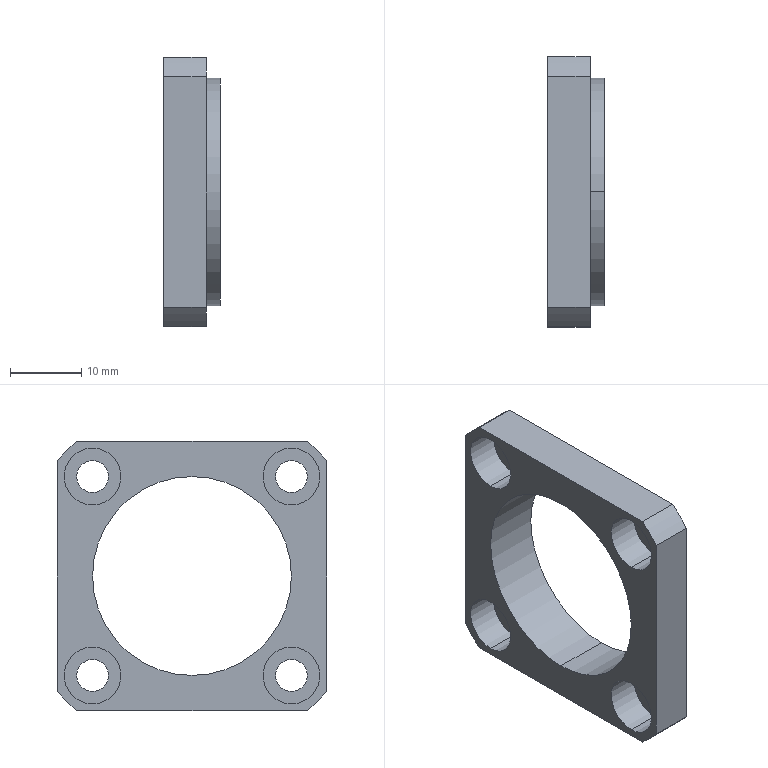Part | STEP file | PN_0056 pressing block | 1 solid | 35 faces | box 8 x 38 x 38 mm | volume 4246 mm3 | cylinder 24 | plane 11 | commonest cylinder face diameters 4.5 x8 8 x8 50 x4 28 x2 32 x2